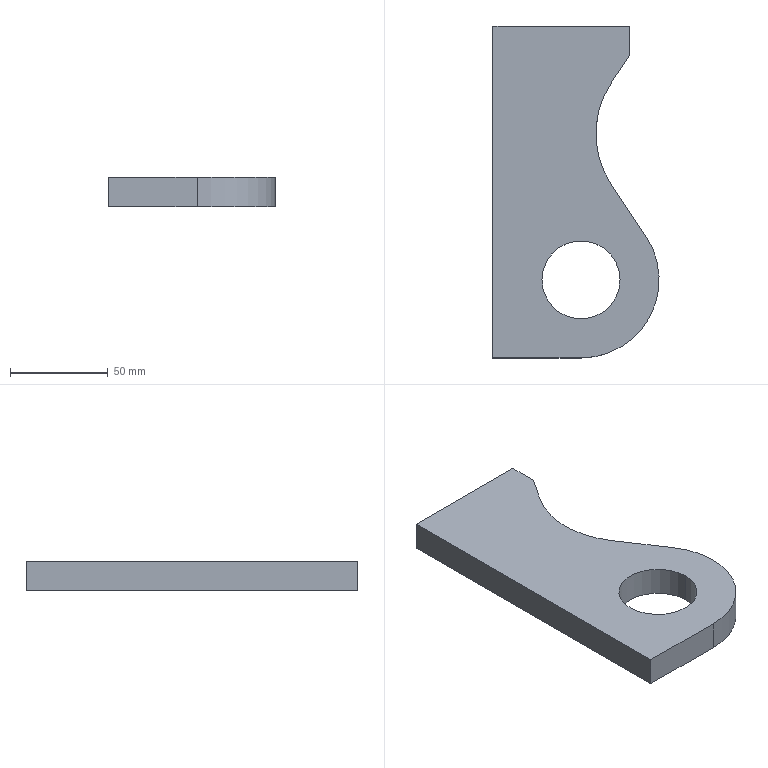Part | SolidWorks | features ICE 3, Extrusion 1 | 1 solid | 12 faces | box 85.082 x 170 x 15 mm | volume 155113 mm3 | plane 8 | cylinder 4 | commonest cylinder face diameters 40 x2 80 x1 93.558 x1
STEP:
#1=CARTESIAN_POINT('',(25.082,-130.,15.));
#2=VERTEX_POINT('',#1);
#3=CARTESIAN_POINT('',(65.082,-130.,15.));
#4=VERTEX_POINT('',#3);
#5=CARTESIAN_POINT('',(45.082,-130.,15.));
#6=DIRECTION('',(0.,0.,1.));
#7=DIRECTION('',(1.,0.,0.));
#8=AXIS2_PLACEMENT_3D('',#5,#6,#7);
#9=CIRCLE('',#8,20.);
#10=EDGE_CURVE('',#2,#4,#9,.T.);
#11=ORIENTED_EDGE('',*,*,#10,.T.);
#12=CARTESIAN_POINT('',(65.082,-130.,0.));
#13=VERTEX_POINT('',#12);
#14=CARTESIAN_POINT('',(65.082,-130.,12.));
#15=DIRECTION('',(0.,0.,-1.));
#16=VECTOR('',#15,1000.);
#17=LINE('',#14,#16);
#18=EDGE_CURVE('',#4,#13,#17,.T.);
#19=ORIENTED_EDGE('',*,*,#18,.T.);
#20=CARTESIAN_POINT('',(25.082,-130.,0.));
#21=VERTEX_POINT('',#20);
#22=CARTESIAN_POINT('',(45.082,-130.,0.));
#23=DIRECTION('',(0.,0.,1.));
#24=DIRECTION('',(1.,0.,0.));
#25=AXIS2_PLACEMENT_3D('',#22,#23,#24);
#26=CIRCLE('',#25,20.);
#27=EDGE_CURVE('',#21,#13,#26,.T.);
#28=ORIENTED_EDGE('',*,*,#27,.F.);
#29=CARTESIAN_POINT('',(25.082,-130.,12.));
#30=DIRECTION('',(0.,0.,-1.));
#31=VECTOR('',#30,1000.);
#32=LINE('',#29,#31);
#33=EDGE_CURVE('',#2,#21,#32,.T.);
#34=ORIENTED_EDGE('',*,*,#33,.F.);
#35=EDGE_LOOP('',(#11,#19,#28,#34));
#36=FACE_OUTER_BOUND('',#35,.T.);
#37=CARTESIAN_POINT('',(45.082,-130.,12.));
#38=DIRECTION('',(0.,0.,-1.));
#39=DIRECTION('',(-1.,0.,0.));
#40=AXIS2_PLACEMENT_3D('',#37,#38,#39);
#41=CYLINDRICAL_SURFACE('',#40,20.);
#42=ADVANCED_FACE('',(#36),#41,.F.);
#43=CARTESIAN_POINT('',(60.544,-29.185,0.));
#44=VERTEX_POINT('',#43);
#45=CARTESIAN_POINT('',(60.544,-29.185,15.));
#46=VERTEX_POINT('',#45);
#47=CARTESIAN_POINT('',(60.544,-29.185,2.));
#48=DIRECTION('',(0.,0.,1.));
#49=VECTOR('',#48,1000.);
#50=LINE('',#47,#49);
#51=EDGE_CURVE('',#44,#46,#50,.T.);
#52=ORIENTED_EDGE('',*,*,#51,.F.);
#53=CARTESIAN_POINT('',(70.,-15.,0.));
#54=VERTEX_POINT('',#53);
#55=CARTESIAN_POINT('',(50.,-45.,0.));
#56=DIRECTION('',(0.5547,0.8321,0.));
#57=VECTOR('',#56,1000.);
#58=LINE('',#55,#57);
#59=EDGE_CURVE('',#44,#54,#58,.T.);
#60=ORIENTED_EDGE('',*,*,#59,.T.);
#61=CARTESIAN_POINT('',(70.,-15.,15.));
#62=VERTEX_POINT('',#61);
#63=CARTESIAN_POINT('',(70.,-15.,12.));
#64=DIRECTION('',(0.,0.,-1.));
#65=VECTOR('',#64,1000.);
#66=LINE('',#63,#65);
#67=EDGE_CURVE('',#62,#54,#66,.T.);
#68=ORIENTED_EDGE('',*,*,#67,.F.);
#69=CARTESIAN_POINT('',(60.544,-29.185,15.));
#70=DIRECTION('',(0.5547,0.8321,0.));
#71=VECTOR('',#70,1000.);
#72=LINE('',#69,#71);
#73=EDGE_CURVE('',#46,#62,#72,.T.);
#74=ORIENTED_EDGE('',*,*,#73,.F.);
#75=EDGE_LOOP('',(#52,#60,#68,#74));
#76=FACE_OUTER_BOUND('',#75,.T.);
#77=CARTESIAN_POINT('',(50.,-45.,12.));
#78=DIRECTION('',(-0.8321,0.5547,0.));
#79=DIRECTION('',(-0.5547,-0.8321,0.));
#80=AXIS2_PLACEMENT_3D('',#77,#78,#79);
#81=PLANE('',#80);
#82=ADVANCED_FACE('',(#76),#81,.F.);
#83=ORIENTED_EDGE('',*,*,#59,.F.);
#84=CARTESIAN_POINT('',(60.544,-81.081,0.));
#85=VERTEX_POINT('',#84);
#86=CARTESIAN_POINT('',(99.466,-55.133,0.));
#87=DIRECTION('',(0.,0.,1.));
#88=DIRECTION('',(-1.,0.,0.));
#89=AXIS2_PLACEMENT_3D('',#86,#87,#88);
#90=CIRCLE('',#89,46.779);
#91=EDGE_CURVE('',#44,#85,#90,.T.);
#92=ORIENTED_EDGE('',*,*,#91,.T.);
#93=CARTESIAN_POINT('',(78.364,-107.812,0.));
#94=VERTEX_POINT('',#93);
#95=CARTESIAN_POINT('',(78.364,-107.812,0.));
#96=DIRECTION('',(-0.5547,0.8321,0.));
#97=VECTOR('',#96,1000.);
#98=LINE('',#95,#97);
#99=EDGE_CURVE('',#94,#85,#98,.T.);
#100=ORIENTED_EDGE('',*,*,#99,.F.);
#101=CARTESIAN_POINT('',(45.082,-170.,0.));
#102=VERTEX_POINT('',#101);
#103=CARTESIAN_POINT('',(45.082,-130.,0.));
#104=DIRECTION('',(0.,0.,1.));
#105=DIRECTION('',(-1.,0.,0.));
#106=AXIS2_PLACEMENT_3D('',#103,#104,#105);
#107=CIRCLE('',#106,40.);
#108=EDGE_CURVE('',#102,#94,#107,.T.);
#109=ORIENTED_EDGE('',*,*,#108,.F.);
#110=CARTESIAN_POINT('',(0.,-170.,0.));
#111=VERTEX_POINT('',#110);
#112=CARTESIAN_POINT('',(0.,-170.,0.));
#113=DIRECTION('',(1.,0.,0.));
#114=VECTOR('',#113,1000.);
#115=LINE('',#112,#114);
#116=EDGE_CURVE('',#111,#102,#115,.T.);
#117=ORIENTED_EDGE('',*,*,#116,.F.);
#118=CARTESIAN_POINT('',(0.,0.,0.));
#119=VERTEX_POINT('',#118);
#120=CARTESIAN_POINT('',(0.,0.,0.));
#121=DIRECTION('',(0.,-1.,0.));
#122=VECTOR('',#121,1000.);
#123=LINE('',#120,#122);
#124=EDGE_CURVE('',#119,#111,#123,.T.);
#125=ORIENTED_EDGE('',*,*,#124,.F.);
#126=CARTESIAN_POINT('',(70.,0.,0.));
#127=VERTEX_POINT('',#126);
#128=CARTESIAN_POINT('',(0.,0.,0.));
#129=DIRECTION('',(-1.,0.,0.));
#130=VECTOR('',#129,1000.);
#131=LINE('',#128,#130);
#132=EDGE_CURVE('',#127,#119,#131,.T.);
#133=ORIENTED_EDGE('',*,*,#132,.F.);
#134=CARTESIAN_POINT('',(70.,0.,0.));
#135=DIRECTION('',(0.,1.,0.));
#136=VECTOR('',#135,1000.);
#137=LINE('',#134,#136);
#138=EDGE_CURVE('',#54,#127,#137,.T.);
#139=ORIENTED_EDGE('',*,*,#138,.F.);
#140=EDGE_LOOP('',(#83,#92,#100,#109,#117,#125,#133,#139));
#141=FACE_OUTER_BOUND('',#140,.T.);
#142=ORIENTED_EDGE('',*,*,#27,.T.);
#143=CARTESIAN_POINT('',(45.082,-130.,0.));
#144=DIRECTION('',(0.,0.,1.));
#145=DIRECTION('',(1.,0.,0.));
#146=AXIS2_PLACEMENT_3D('',#143,#144,#145);
#147=CIRCLE('',#146,20.);
#148=EDGE_CURVE('',#13,#21,#147,.T.);
#149=ORIENTED_EDGE('',*,*,#148,.T.);
#150=EDGE_LOOP('',(#142,#149));
#151=FACE_BOUND('',#150,.T.);
#152=CARTESIAN_POINT('',(45.082,-130.,0.));
#153=DIRECTION('',(0.,0.,-1.));
#154=DIRECTION('',(-1.,0.,0.));
#155=AXIS2_PLACEMENT_3D('',#152,#153,#154);
#156=PLANE('',#155);
#157=ADVANCED_FACE('',(#141,#151),#156,.T.);
#158=ORIENTED_EDGE('',*,*,#124,.T.);
#159=CARTESIAN_POINT('',(0.,-170.,15.));
#160=VERTEX_POINT('',#159);
#161=CARTESIAN_POINT('',(0.,-170.,12.));
#162=DIRECTION('',(0.,0.,-1.));
#163=VECTOR('',#162,1000.);
#164=LINE('',#161,#163);
#165=EDGE_CURVE('',#160,#111,#164,.T.);
#166=ORIENTED_EDGE('',*,*,#165,.F.);
#167=CARTESIAN_POINT('',(0.,0.,15.));
#168=VERTEX_POINT('',#167);
#169=CARTESIAN_POINT('',(0.,0.,15.));
#170=DIRECTION('',(0.,-1.,0.));
#171=VECTOR('',#170,1000.);
#172=LINE('',#169,#171);
#173=EDGE_CURVE('',#168,#160,#172,.T.);
#174=ORIENTED_EDGE('',*,*,#173,.F.);
#175=CARTESIAN_POINT('',(0.,0.,12.));
#176=DIRECTION('',(0.,0.,-1.));
#177=VECTOR('',#176,1000.);
#178=LINE('',#175,#177);
#179=EDGE_CURVE('',#168,#119,#178,.T.);
#180=ORIENTED_EDGE('',*,*,#179,.T.);
#181=EDGE_LOOP('',(#158,#166,#174,#180));
#182=FACE_OUTER_BOUND('',#181,.T.);
#183=CARTESIAN_POINT('',(0.,0.,12.));
#184=DIRECTION('',(1.,0.,0.));
#185=DIRECTION('',(0.,1.,0.));
#186=AXIS2_PLACEMENT_3D('',#183,#184,#185);
#187=PLANE('',#186);
#188=ADVANCED_FACE('',(#182),#187,.F.);
#189=ORIENTED_EDGE('',*,*,#116,.T.);
#190=CARTESIAN_POINT('',(45.082,-170.,15.));
#191=VERTEX_POINT('',#190);
#192=CARTESIAN_POINT('',(45.082,-170.,12.));
#193=DIRECTION('',(0.,0.,-1.));
#194=VECTOR('',#193,1000.);
#195=LINE('',#192,#194);
#196=EDGE_CURVE('',#191,#102,#195,.T.);
#197=ORIENTED_EDGE('',*,*,#196,.F.);
#198=CARTESIAN_POINT('',(0.,-170.,15.));
#199=DIRECTION('',(1.,0.,0.));
#200=VECTOR('',#199,1000.);
#201=LINE('',#198,#200);
#202=EDGE_CURVE('',#160,#191,#201,.T.);
#203=ORIENTED_EDGE('',*,*,#202,.F.);
#204=ORIENTED_EDGE('',*,*,#165,.T.);
#205=EDGE_LOOP('',(#189,#197,#203,#204));
#206=FACE_OUTER_BOUND('',#205,.T.);
#207=CARTESIAN_POINT('',(0.,-170.,12.));
#208=DIRECTION('',(0.,1.,0.));
#209=DIRECTION('',(0.,0.,1.));
#210=AXIS2_PLACEMENT_3D('',#207,#208,#209);
#211=PLANE('',#210);
#212=ADVANCED_FACE('',(#206),#211,.F.);
#213=ORIENTED_EDGE('',*,*,#108,.T.);
#214=CARTESIAN_POINT('',(78.364,-107.812,15.));
#215=VERTEX_POINT('',#214);
#216=CARTESIAN_POINT('',(78.364,-107.812,12.));
#217=DIRECTION('',(0.,0.,-1.));
#218=VECTOR('',#217,1000.);
#219=LINE('',#216,#218);
#220=EDGE_CURVE('',#215,#94,#219,.T.);
#221=ORIENTED_EDGE('',*,*,#220,.F.);
#222=CARTESIAN_POINT('',(45.082,-130.,15.));
#223=DIRECTION('',(0.,0.,1.));
#224=DIRECTION('',(1.,0.,0.));
#225=AXIS2_PLACEMENT_3D('',#222,#223,#224);
#226=CIRCLE('',#225,40.);
#227=EDGE_CURVE('',#191,#215,#226,.T.);
#228=ORIENTED_EDGE('',*,*,#227,.F.);
#229=ORIENTED_EDGE('',*,*,#196,.T.);
#230=EDGE_LOOP('',(#213,#221,#228,#229));
#231=FACE_OUTER_BOUND('',#230,.T.);
#232=CARTESIAN_POINT('',(45.082,-130.,12.));
#233=DIRECTION('',(0.,0.,-1.));
#234=DIRECTION('',(-1.,0.,0.));
#235=AXIS2_PLACEMENT_3D('',#232,#233,#234);
#236=CYLINDRICAL_SURFACE('',#235,40.);
#237=ADVANCED_FACE('',(#231),#236,.T.);
#238=ORIENTED_EDGE('',*,*,#99,.T.);
#239=CARTESIAN_POINT('',(60.544,-81.081,15.));
#240=VERTEX_POINT('',#239);
#241=CARTESIAN_POINT('',(60.544,-81.081,2.));
#242=DIRECTION('',(0.,0.,1.));
#243=VECTOR('',#242,1000.);
#244=LINE('',#241,#243);
#245=EDGE_CURVE('',#85,#240,#244,.T.);
#246=ORIENTED_EDGE('',*,*,#245,.T.);
#247=CARTESIAN_POINT('',(78.364,-107.812,15.));
#248=DIRECTION('',(-0.5547,0.8321,0.));
#249=VECTOR('',#248,1000.);
#250=LINE('',#247,#249);
#251=EDGE_CURVE('',#215,#240,#250,.T.);
#252=ORIENTED_EDGE('',*,*,#251,.F.);
#253=ORIENTED_EDGE('',*,*,#220,.T.);
#254=EDGE_LOOP('',(#238,#246,#252,#253));
#255=FACE_OUTER_BOUND('',#254,.T.);
#256=CARTESIAN_POINT('',(78.364,-107.812,12.));
#257=DIRECTION('',(-0.8321,-0.5547,0.));
#258=DIRECTION('',(0.5547,-0.8321,0.));
#259=AXIS2_PLACEMENT_3D('',#256,#257,#258);
#260=PLANE('',#259);
#261=ADVANCED_FACE('',(#255),#260,.F.);
#262=ORIENTED_EDGE('',*,*,#138,.T.);
#263=CARTESIAN_POINT('',(70.,0.,15.));
#264=VERTEX_POINT('',#263);
#265=CARTESIAN_POINT('',(70.,0.,12.));
#266=DIRECTION('',(0.,0.,-1.));
#267=VECTOR('',#266,1000.);
#268=LINE('',#265,#267);
#269=EDGE_CURVE('',#264,#127,#268,.T.);
#270=ORIENTED_EDGE('',*,*,#269,.F.);
#271=CARTESIAN_POINT('',(70.,-15.,15.));
#272=DIRECTION('',(0.,1.,0.));
#273=VECTOR('',#272,1000.);
#274=LINE('',#271,#273);
#275=EDGE_CURVE('',#62,#264,#274,.T.);
#276=ORIENTED_EDGE('',*,*,#275,.F.);
#277=ORIENTED_EDGE('',*,*,#67,.T.);
#278=EDGE_LOOP('',(#262,#270,#276,#277));
#279=FACE_OUTER_BOUND('',#278,.T.);
#280=CARTESIAN_POINT('',(70.,0.,12.));
#281=DIRECTION('',(-1.,0.,0.));
#282=DIRECTION('',(0.,0.,1.));
#283=AXIS2_PLACEMENT_3D('',#280,#281,#282);
#284=PLANE('',#283);
#285=ADVANCED_FACE('',(#279),#284,.F.);
#286=ORIENTED_EDGE('',*,*,#132,.T.);
#287=ORIENTED_EDGE('',*,*,#179,.F.);
#288=CARTESIAN_POINT('',(70.,0.,15.));
#289=DIRECTION('',(-1.,0.,0.));
#290=VECTOR('',#289,1000.);
#291=LINE('',#288,#290);
#292=EDGE_CURVE('',#264,#168,#291,.T.);
#293=ORIENTED_EDGE('',*,*,#292,.F.);
#294=ORIENTED_EDGE('',*,*,#269,.T.);
#295=EDGE_LOOP('',(#286,#287,#293,#294));
#296=FACE_OUTER_BOUND('',#295,.T.);
#297=CARTESIAN_POINT('',(0.,0.,12.));
#298=DIRECTION('',(0.,-1.,0.));
#299=DIRECTION('',(0.,0.,-1.));
#300=AXIS2_PLACEMENT_3D('',#297,#298,#299);
#301=PLANE('',#300);
#302=ADVANCED_FACE('',(#296),#301,.F.);
#303=ORIENTED_EDGE('',*,*,#18,.F.);
#304=CARTESIAN_POINT('',(45.082,-130.,15.));
#305=DIRECTION('',(0.,0.,1.));
#306=DIRECTION('',(1.,0.,0.));
#307=AXIS2_PLACEMENT_3D('',#304,#305,#306);
#308=CIRCLE('',#307,20.);
#309=EDGE_CURVE('',#4,#2,#308,.T.);
#310=ORIENTED_EDGE('',*,*,#309,.T.);
#311=ORIENTED_EDGE('',*,*,#33,.T.);
#312=ORIENTED_EDGE('',*,*,#148,.F.);
#313=EDGE_LOOP('',(#303,#310,#311,#312));
#314=FACE_OUTER_BOUND('',#313,.T.);
#315=CARTESIAN_POINT('',(45.082,-130.,12.));
#316=DIRECTION('',(0.,0.,-1.));
#317=DIRECTION('',(-1.,0.,0.));
#318=AXIS2_PLACEMENT_3D('',#315,#316,#317);
#319=CYLINDRICAL_SURFACE('',#318,20.);
#320=ADVANCED_FACE('',(#314),#319,.F.);
#321=ORIENTED_EDGE('',*,*,#51,.T.);
#322=CARTESIAN_POINT('',(99.466,-55.133,15.));
#323=DIRECTION('',(0.,0.,-1.));
#324=DIRECTION('',(1.,0.,0.));
#325=AXIS2_PLACEMENT_3D('',#322,#323,#324);
#326=CIRCLE('',#325,46.779);
#327=EDGE_CURVE('',#240,#46,#326,.T.);
#328=ORIENTED_EDGE('',*,*,#327,.F.);
#329=ORIENTED_EDGE('',*,*,#245,.F.);
#330=ORIENTED_EDGE('',*,*,#91,.F.);
#331=EDGE_LOOP('',(#321,#328,#329,#330));
#332=FACE_OUTER_BOUND('',#331,.T.);
#333=CARTESIAN_POINT('',(99.466,-55.133,2.));
#334=DIRECTION('',(0.,0.,1.));
#335=DIRECTION('',(1.,0.,0.));
#336=AXIS2_PLACEMENT_3D('',#333,#334,#335);
#337=CYLINDRICAL_SURFACE('',#336,46.779);
#338=ADVANCED_FACE('',(#332),#337,.F.);
#339=ORIENTED_EDGE('',*,*,#292,.T.);
#340=ORIENTED_EDGE('',*,*,#173,.T.);
#341=ORIENTED_EDGE('',*,*,#202,.T.);
#342=ORIENTED_EDGE('',*,*,#227,.T.);
#343=ORIENTED_EDGE('',*,*,#251,.T.);
#344=ORIENTED_EDGE('',*,*,#327,.T.);
#345=ORIENTED_EDGE('',*,*,#73,.T.);
#346=ORIENTED_EDGE('',*,*,#275,.T.);
#347=EDGE_LOOP('',(#339,#340,#341,#342,#343,#344,#345,#346));
#348=FACE_OUTER_BOUND('',#347,.T.);
#349=ORIENTED_EDGE('',*,*,#10,.F.);
#350=ORIENTED_EDGE('',*,*,#309,.F.);
#351=EDGE_LOOP('',(#349,#350));
#352=FACE_BOUND('',#351,.T.);
#353=CARTESIAN_POINT('',(45.082,-130.,15.));
#354=DIRECTION('',(0.,0.,1.));
#355=DIRECTION('',(1.,0.,0.));
#356=AXIS2_PLACEMENT_3D('',#353,#354,#355);
#357=PLANE('',#356);
#358=ADVANCED_FACE('',(#348,#352),#357,.T.);
#359=CLOSED_SHELL('',(#42,#82,#157,#188,#212,#237,#261,#285,#302,#320,#338,#358));
#360=MANIFOLD_SOLID_BREP('',#359);
#361=CARTESIAN_POINT('',(0.,0.,0.));
#362=DIRECTION('',(0.,0.,1.));
#363=DIRECTION('',(1.,0.,0.));
#364=AXIS2_PLACEMENT_3D('',#361,#362,#363);
#365=(LENGTH_UNIT()NAMED_UNIT(*)SI_UNIT(.MILLI.,.METRE.));
#366=UNCERTAINTY_MEASURE_WITH_UNIT(LENGTH_MEASURE(0.00001),#365,'','');
#367=(NAMED_UNIT(*)PLANE_ANGLE_UNIT()SI_UNIT($,.RADIAN.));
#368=(NAMED_UNIT(*)SI_UNIT($,.STERADIAN.)SOLID_ANGLE_UNIT());
#369=(GEOMETRIC_REPRESENTATION_CONTEXT(3)GLOBAL_UNCERTAINTY_ASSIGNED_CONTEXT((#366))GLOBAL_UNIT_ASSIGNED_CONTEXT((#365,#367,#368))REPRESENTATION_CONTEXT('',''));
#370=ADVANCED_BREP_SHAPE_REPRESENTATION('',(#360,#364),#369);